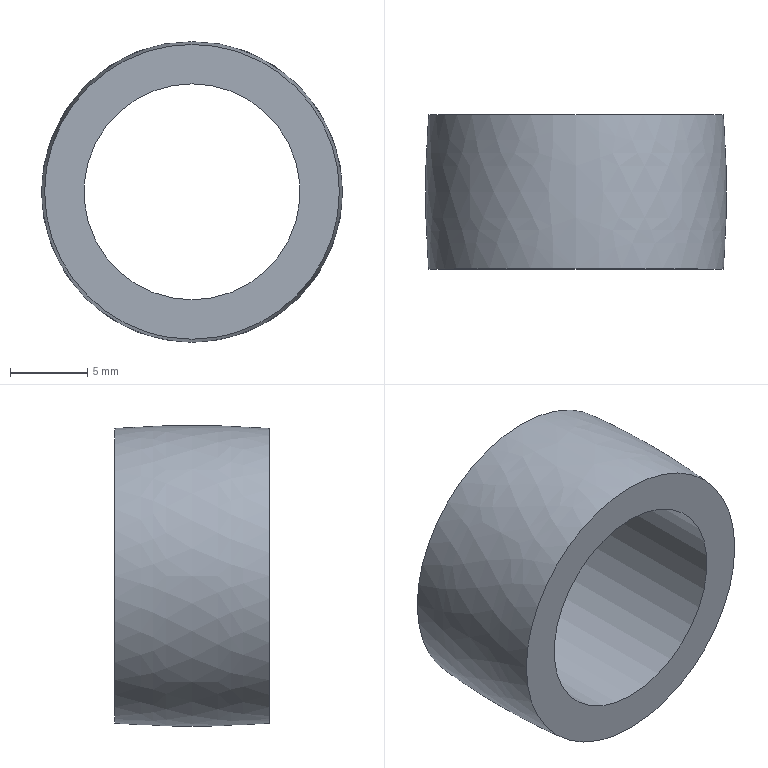Part | STEP file | 1-46.12 | 1 solid | 4 faces | box 19.5 x 10 x 19.5 mm | volume 1406 mm3 | plane 2 | cylinder 1 | spline 1 | commonest cylinder face diameters 14 x1
STEP:
#1=CARTESIAN_POINT('',(0.,0.,0.));
#2=DIRECTION('',(0.,0.,1.));
#3=DIRECTION('',(1.,0.,0.));
#4=AXIS2_PLACEMENT_3D('',#1,#2,#3);
#5=CARTESIAN_POINT('',(0.,0.,7.));
#6=VERTEX_POINT('',#5);
#7=CARTESIAN_POINT('',(0.,0.,0.));
#8=DIRECTION('',(0.,1.,0.));
#9=DIRECTION('',(0.,0.,1.));
#10=AXIS2_PLACEMENT_3D('',#7,#8,#9);
#11=CIRCLE('',#10,7.);
#12=CARTESIAN_POINT('',(0.,0.,0.));
#13=DIRECTION('',(0.,1.,0.));
#14=DIRECTION('',(0.,0.,1.));
#15=AXIS2_PLACEMENT_3D('',#12,#13,#14);
#16=CYLINDRICAL_SURFACE('',#15,7.);
#17=CARTESIAN_POINT('',(0.,0.));
#18=DIRECTION('',(1.,0.));
#19=VECTOR('',#18,1.);
#20=LINE('',#17,#19);
#21=(GEOMETRIC_REPRESENTATION_CONTEXT(2)PARAMETRIC_REPRESENTATION_CONTEXT()REPRESENTATION_CONTEXT('',''));
#22=DEFINITIONAL_REPRESENTATION('',(#20),#21);
#23=PCURVE('',#16,#22);
#24=CARTESIAN_POINT('',(0.,0.,0.));
#25=DIRECTION('',(0.,-1.,0.));
#26=DIRECTION('',(0.,0.,1.));
#27=AXIS2_PLACEMENT_3D('',#24,#25,#26);
#28=PLANE('',#27);
#29=CARTESIAN_POINT('',(7.,0.));
#30=CARTESIAN_POINT('',(7.,-12.124));
#31=CARTESIAN_POINT('',(-3.5,-6.062));
#32=CARTESIAN_POINT('',(-14.,0.));
#33=CARTESIAN_POINT('',(-3.5,6.062));
#34=CARTESIAN_POINT('',(7.,12.124));
#35=CARTESIAN_POINT('',(7.,0.));
#36=(BOUNDED_CURVE()B_SPLINE_CURVE(2,(#29,#30,#31,#32,#33,#34,#35),.UNSPECIFIED.,.T.,.F.)B_SPLINE_CURVE_WITH_KNOTS((1,2,2,2,2,1),(-2.094,0.,2.094,4.189,6.283,8.378),.UNSPECIFIED.)CURVE()GEOMETRIC_REPRESENTATION_ITEM()RATIONAL_B_SPLINE_CURVE((1.,0.5,1.,0.5,1.,0.5,1.))REPRESENTATION_ITEM(''));
#37=(GEOMETRIC_REPRESENTATION_CONTEXT(2)PARAMETRIC_REPRESENTATION_CONTEXT()REPRESENTATION_CONTEXT('',''));
#38=DEFINITIONAL_REPRESENTATION('',(#36),#37);
#39=PCURVE('',#28,#38);
#40=SURFACE_CURVE('',#11,(#23,#39),.PCURVE_S1.);
#41=EDGE_CURVE('',#6,#6,#40,.T.);
#42=ORIENTED_EDGE('',*,*,#41,.T.);
#43=CARTESIAN_POINT('',(0.,10.,7.));
#44=VERTEX_POINT('',#43);
#45=CARTESIAN_POINT('',(0.,0.,7.));
#46=DIRECTION('',(0.,1.,0.));
#47=VECTOR('',#46,1.);
#48=LINE('',#45,#47);
#49=CARTESIAN_POINT('',(6.283,0.));
#50=DIRECTION('',(0.,1.));
#51=VECTOR('',#50,1.);
#52=LINE('',#49,#51);
#53=(GEOMETRIC_REPRESENTATION_CONTEXT(2)PARAMETRIC_REPRESENTATION_CONTEXT()REPRESENTATION_CONTEXT('',''));
#54=DEFINITIONAL_REPRESENTATION('',(#52),#53);
#55=PCURVE('',#16,#54);
#56=CARTESIAN_POINT('',(0.,0.));
#57=DIRECTION('',(0.,1.));
#58=VECTOR('',#57,1.);
#59=LINE('',#56,#58);
#60=(GEOMETRIC_REPRESENTATION_CONTEXT(2)PARAMETRIC_REPRESENTATION_CONTEXT()REPRESENTATION_CONTEXT('',''));
#61=DEFINITIONAL_REPRESENTATION('',(#59),#60);
#62=PCURVE('',#16,#61);
#63=SEAM_CURVE('',#48,(#55,#62),.PCURVE_S1.);
#64=EDGE_CURVE('',#6,#44,#63,.T.);
#65=ORIENTED_EDGE('',*,*,#64,.T.);
#66=CARTESIAN_POINT('',(0.,10.,0.));
#67=DIRECTION('',(0.,1.,0.));
#68=DIRECTION('',(0.,0.,1.));
#69=AXIS2_PLACEMENT_3D('',#66,#67,#68);
#70=CIRCLE('',#69,7.);
#71=CARTESIAN_POINT('',(0.,10.));
#72=DIRECTION('',(1.,0.));
#73=VECTOR('',#72,1.);
#74=LINE('',#71,#73);
#75=(GEOMETRIC_REPRESENTATION_CONTEXT(2)PARAMETRIC_REPRESENTATION_CONTEXT()REPRESENTATION_CONTEXT('',''));
#76=DEFINITIONAL_REPRESENTATION('',(#74),#75);
#77=PCURVE('',#16,#76);
#78=CARTESIAN_POINT('',(0.,10.,0.));
#79=DIRECTION('',(0.,1.,0.));
#80=DIRECTION('',(0.,0.,1.));
#81=AXIS2_PLACEMENT_3D('',#78,#79,#80);
#82=PLANE('',#81);
#83=CARTESIAN_POINT('',(0.,0.));
#84=DIRECTION('',(1.,0.));
#85=AXIS2_PLACEMENT_2D('',#83,#84);
#86=CIRCLE('',#85,7.);
#87=(GEOMETRIC_REPRESENTATION_CONTEXT(2)PARAMETRIC_REPRESENTATION_CONTEXT()REPRESENTATION_CONTEXT('',''));
#88=DEFINITIONAL_REPRESENTATION('',(#86),#87);
#89=PCURVE('',#82,#88);
#90=SURFACE_CURVE('',#70,(#77,#89),.PCURVE_S1.);
#91=EDGE_CURVE('',#44,#44,#90,.T.);
#92=ORIENTED_EDGE('',*,*,#91,.F.);
#93=ORIENTED_EDGE('',*,*,#64,.F.);
#94=EDGE_LOOP('',(#42,#65,#92,#93));
#95=FACE_BOUND('',#94,.F.);
#96=ADVANCED_FACE('',(#95),#16,.F.);
#97=CARTESIAN_POINT('',(0.,10.,9.55));
#98=VERTEX_POINT('',#97);
#99=CARTESIAN_POINT('',(0.,10.,0.));
#100=DIRECTION('',(0.,1.,0.));
#101=DIRECTION('',(0.,0.,1.));
#102=AXIS2_PLACEMENT_3D('',#99,#100,#101);
#103=CIRCLE('',#102,9.55);
#104=CARTESIAN_POINT('',(0.,0.));
#105=DIRECTION('',(1.,0.));
#106=AXIS2_PLACEMENT_2D('',#104,#105);
#107=CIRCLE('',#106,9.55);
#108=(GEOMETRIC_REPRESENTATION_CONTEXT(2)PARAMETRIC_REPRESENTATION_CONTEXT()REPRESENTATION_CONTEXT('',''));
#109=DEFINITIONAL_REPRESENTATION('',(#107),#108);
#110=PCURVE('',#82,#109);
#111=CARTESIAN_POINT('',(0.,10.,9.55));
#112=CARTESIAN_POINT('',(9.55,10.,9.55));
#113=CARTESIAN_POINT('',(9.55,10.,0.));
#114=CARTESIAN_POINT('',(9.55,10.,-9.55));
#115=CARTESIAN_POINT('',(0.,10.,-9.55));
#116=CARTESIAN_POINT('',(-9.55,10.,-9.55));
#117=CARTESIAN_POINT('',(-9.55,10.,0.));
#118=CARTESIAN_POINT('',(-9.55,10.,9.55));
#119=CARTESIAN_POINT('',(0.,10.,9.55));
#120=CARTESIAN_POINT('',(0.,5.,9.951));
#121=CARTESIAN_POINT('',(9.951,5.,9.951));
#122=CARTESIAN_POINT('',(9.951,5.,0.));
#123=CARTESIAN_POINT('',(9.951,5.,-9.951));
#124=CARTESIAN_POINT('',(0.,5.,-9.951));
#125=CARTESIAN_POINT('',(-9.951,5.,-9.951));
#126=CARTESIAN_POINT('',(-9.951,5.,0.));
#127=CARTESIAN_POINT('',(-9.951,5.,9.951));
#128=CARTESIAN_POINT('',(0.,5.,9.951));
#129=CARTESIAN_POINT('',(0.,0.,9.55));
#130=CARTESIAN_POINT('',(9.55,0.,9.55));
#131=CARTESIAN_POINT('',(9.55,0.,0.));
#132=CARTESIAN_POINT('',(9.55,0.,-9.55));
#133=CARTESIAN_POINT('',(0.,0.,-9.55));
#134=CARTESIAN_POINT('',(-9.55,0.,-9.55));
#135=CARTESIAN_POINT('',(-9.55,0.,0.));
#136=CARTESIAN_POINT('',(-9.55,0.,9.55));
#137=CARTESIAN_POINT('',(0.,0.,9.55));
#138=(BOUNDED_SURFACE()B_SPLINE_SURFACE(2,2,((#111,#112,#113,#114,#115,#116,#117,#118,#119),(#120,#121,#122,#123,#124,#125,#126,#127,#128),(#129,#130,#131,#132,#133,#134,#135,#136,#137)),.UNSPECIFIED.,.F.,.T.,.F.)B_SPLINE_SURFACE_WITH_KNOTS((3,3),(1,2,2,2,2,2,1),(0.,1.),(-0.25,0.,0.25,0.5,0.75,1.,1.25),.UNSPECIFIED.)GEOMETRIC_REPRESENTATION_ITEM()RATIONAL_B_SPLINE_SURFACE(((1.,0.7071,1.,0.7071,1.,0.7071,1.,0.7071,1.),(0.9968,0.7048,0.9968,0.7048,0.9968,0.7048,0.9968,0.7048,0.9968),(1.,0.7071,1.,0.7071,1.,0.7071,1.,0.7071,1.)))REPRESENTATION_ITEM('')SURFACE());
#139=CARTESIAN_POINT('',(0.,0.));
#140=CARTESIAN_POINT('',(0.,0.01678));
#141=CARTESIAN_POINT('',(0.,0.04854));
#142=CARTESIAN_POINT('',(0.,0.09277));
#143=CARTESIAN_POINT('',(0.,0.1357));
#144=CARTESIAN_POINT('',(0.,0.1791));
#145=CARTESIAN_POINT('',(0.,0.2245));
#146=CARTESIAN_POINT('',(0.,0.2755));
#147=CARTESIAN_POINT('',(0.,0.3209));
#148=CARTESIAN_POINT('',(0.,0.3643));
#149=CARTESIAN_POINT('',(0.,0.4073));
#150=CARTESIAN_POINT('',(0.,0.4512));
#151=CARTESIAN_POINT('',(0.,0.5));
#152=CARTESIAN_POINT('',(0.,0.5488));
#153=CARTESIAN_POINT('',(0.,0.5927));
#154=CARTESIAN_POINT('',(0.,0.6357));
#155=CARTESIAN_POINT('',(0.,0.6791));
#156=CARTESIAN_POINT('',(0.,0.7245));
#157=CARTESIAN_POINT('',(0.,0.7755));
#158=CARTESIAN_POINT('',(0.,0.8209));
#159=CARTESIAN_POINT('',(0.,0.8643));
#160=CARTESIAN_POINT('',(0.,0.9072));
#161=CARTESIAN_POINT('',(0.,0.9515));
#162=CARTESIAN_POINT('',(0.,0.9832));
#163=CARTESIAN_POINT('',(0.,1.));
#164=B_SPLINE_CURVE_WITH_KNOTS('',3,(#139,#140,#141,#142,#143,#144,#145,#146,#147,#148,#149,#150,#151,#152,#153,#154,#155,#156,#157,#158,#159,#160,#161,#162,#163),.UNSPECIFIED.,.F.,.F.,(4,1,1,1,1,1,1,1,1,1,1,1,1,1,1,1,1,1,1,1,1,1,4),(0.,0.2856,0.5712,0.8568,1.142,1.428,1.714,1.999,2.285,2.57,2.856,3.142,3.427,3.713,3.998,4.284,4.57,4.855,5.141,5.426,5.712,5.998,6.283),.QUASI_UNIFORM_KNOTS.);
#165=(GEOMETRIC_REPRESENTATION_CONTEXT(2)PARAMETRIC_REPRESENTATION_CONTEXT()REPRESENTATION_CONTEXT('',''));
#166=DEFINITIONAL_REPRESENTATION('',(#164),#165);
#167=PCURVE('',#138,#166);
#168=SURFACE_CURVE('',#103,(#110,#167),.PCURVE_S1.);
#169=EDGE_CURVE('',#98,#98,#168,.T.);
#170=ORIENTED_EDGE('',*,*,#169,.T.);
#171=EDGE_LOOP('',(#170));
#172=FACE_BOUND('',#171,.T.);
#173=ORIENTED_EDGE('',*,*,#91,.F.);
#174=EDGE_LOOP('',(#173));
#175=FACE_BOUND('',#174,.T.);
#176=ADVANCED_FACE('',(#172,#175),#82,.T.);
#177=CARTESIAN_POINT('',(0.,0.,9.55));
#178=VERTEX_POINT('',#177);
#179=CARTESIAN_POINT('',(0.,5.,-52.85));
#180=DIRECTION('',(1.,0.,0.));
#181=DIRECTION('',(0.,0.07987,0.9968));
#182=AXIS2_PLACEMENT_3D('',#179,#180,#181);
#183=CIRCLE('',#182,62.6);
#184=CARTESIAN_POINT('',(0.,0.));
#185=CARTESIAN_POINT('',(1.,0.));
#186=B_SPLINE_CURVE_WITH_KNOTS('',1,(#184,#185),.UNSPECIFIED.,.F.,.F.,(2,2),(0.,0.1599),.PIECEWISE_BEZIER_KNOTS.);
#187=(GEOMETRIC_REPRESENTATION_CONTEXT(2)PARAMETRIC_REPRESENTATION_CONTEXT()REPRESENTATION_CONTEXT('',''));
#188=DEFINITIONAL_REPRESENTATION('',(#186),#187);
#189=PCURVE('',#138,#188);
#190=CARTESIAN_POINT('',(0.,1.));
#191=CARTESIAN_POINT('',(1.,1.));
#192=B_SPLINE_CURVE_WITH_KNOTS('',1,(#190,#191),.UNSPECIFIED.,.F.,.F.,(2,2),(0.,0.1599),.PIECEWISE_BEZIER_KNOTS.);
#193=(GEOMETRIC_REPRESENTATION_CONTEXT(2)PARAMETRIC_REPRESENTATION_CONTEXT()REPRESENTATION_CONTEXT('',''));
#194=DEFINITIONAL_REPRESENTATION('',(#192),#193);
#195=PCURVE('',#138,#194);
#196=SEAM_CURVE('',#183,(#189,#195),.PCURVE_S1.);
#197=EDGE_CURVE('',#98,#178,#196,.T.);
#198=ORIENTED_EDGE('',*,*,#197,.T.);
#199=CARTESIAN_POINT('',(0.,0.,0.));
#200=DIRECTION('',(0.,1.,0.));
#201=DIRECTION('',(0.,0.,1.));
#202=AXIS2_PLACEMENT_3D('',#199,#200,#201);
#203=CIRCLE('',#202,9.55);
#204=CARTESIAN_POINT('',(1.,0.));
#205=CARTESIAN_POINT('',(1.,0.01678));
#206=CARTESIAN_POINT('',(1.,0.04854));
#207=CARTESIAN_POINT('',(1.,0.09277));
#208=CARTESIAN_POINT('',(1.,0.1357));
#209=CARTESIAN_POINT('',(1.,0.1791));
#210=CARTESIAN_POINT('',(1.,0.2245));
#211=CARTESIAN_POINT('',(1.,0.2755));
#212=CARTESIAN_POINT('',(1.,0.3209));
#213=CARTESIAN_POINT('',(1.,0.3643));
#214=CARTESIAN_POINT('',(1.,0.4073));
#215=CARTESIAN_POINT('',(1.,0.4512));
#216=CARTESIAN_POINT('',(1.,0.5));
#217=CARTESIAN_POINT('',(1.,0.5488));
#218=CARTESIAN_POINT('',(1.,0.5927));
#219=CARTESIAN_POINT('',(1.,0.6357));
#220=CARTESIAN_POINT('',(1.,0.6791));
#221=CARTESIAN_POINT('',(1.,0.7245));
#222=CARTESIAN_POINT('',(1.,0.7755));
#223=CARTESIAN_POINT('',(1.,0.8209));
#224=CARTESIAN_POINT('',(1.,0.8643));
#225=CARTESIAN_POINT('',(1.,0.9072));
#226=CARTESIAN_POINT('',(1.,0.9515));
#227=CARTESIAN_POINT('',(1.,0.9832));
#228=CARTESIAN_POINT('',(1.,1.));
#229=B_SPLINE_CURVE_WITH_KNOTS('',3,(#204,#205,#206,#207,#208,#209,#210,#211,#212,#213,#214,#215,#216,#217,#218,#219,#220,#221,#222,#223,#224,#225,#226,#227,#228),.UNSPECIFIED.,.F.,.F.,(4,1,1,1,1,1,1,1,1,1,1,1,1,1,1,1,1,1,1,1,1,1,4),(0.,0.2856,0.5712,0.8568,1.142,1.428,1.714,1.999,2.285,2.57,2.856,3.142,3.427,3.713,3.998,4.284,4.57,4.855,5.141,5.426,5.712,5.998,6.283),.QUASI_UNIFORM_KNOTS.);
#230=(GEOMETRIC_REPRESENTATION_CONTEXT(2)PARAMETRIC_REPRESENTATION_CONTEXT()REPRESENTATION_CONTEXT('',''));
#231=DEFINITIONAL_REPRESENTATION('',(#229),#230);
#232=PCURVE('',#138,#231);
#233=CARTESIAN_POINT('',(9.55,0.));
#234=CARTESIAN_POINT('',(9.55,-16.541));
#235=CARTESIAN_POINT('',(-4.775,-8.271));
#236=CARTESIAN_POINT('',(-19.1,0.));
#237=CARTESIAN_POINT('',(-4.775,8.271));
#238=CARTESIAN_POINT('',(9.55,16.541));
#239=CARTESIAN_POINT('',(9.55,0.));
#240=(BOUNDED_CURVE()B_SPLINE_CURVE(2,(#233,#234,#235,#236,#237,#238,#239),.UNSPECIFIED.,.T.,.F.)B_SPLINE_CURVE_WITH_KNOTS((1,2,2,2,2,1),(-2.094,0.,2.094,4.189,6.283,8.378),.UNSPECIFIED.)CURVE()GEOMETRIC_REPRESENTATION_ITEM()RATIONAL_B_SPLINE_CURVE((1.,0.5,1.,0.5,1.,0.5,1.))REPRESENTATION_ITEM(''));
#241=(GEOMETRIC_REPRESENTATION_CONTEXT(2)PARAMETRIC_REPRESENTATION_CONTEXT()REPRESENTATION_CONTEXT('',''));
#242=DEFINITIONAL_REPRESENTATION('',(#240),#241);
#243=PCURVE('',#28,#242);
#244=SURFACE_CURVE('',#203,(#232,#243),.PCURVE_S1.);
#245=EDGE_CURVE('',#178,#178,#244,.T.);
#246=ORIENTED_EDGE('',*,*,#245,.T.);
#247=ORIENTED_EDGE('',*,*,#197,.F.);
#248=ORIENTED_EDGE('',*,*,#169,.F.);
#249=EDGE_LOOP('',(#198,#246,#247,#248));
#250=FACE_BOUND('',#249,.T.);
#251=ADVANCED_FACE('',(#250),#138,.T.);
#252=ORIENTED_EDGE('',*,*,#245,.F.);
#253=EDGE_LOOP('',(#252));
#254=FACE_BOUND('',#253,.T.);
#255=ORIENTED_EDGE('',*,*,#41,.T.);
#256=EDGE_LOOP('',(#255));
#257=FACE_BOUND('',#256,.T.);
#258=ADVANCED_FACE('',(#254,#257),#28,.T.);
#259=CLOSED_SHELL('',(#96,#176,#251,#258));
#260=MANIFOLD_SOLID_BREP('',#259);
#261=(LENGTH_UNIT()NAMED_UNIT(*)SI_UNIT(.MILLI.,.METRE.));
#262=UNCERTAINTY_MEASURE_WITH_UNIT(LENGTH_MEASURE(0.0005),#261,'','');
#263=(NAMED_UNIT(*)PLANE_ANGLE_UNIT()SI_UNIT($,.RADIAN.));
#264=(NAMED_UNIT(*)SI_UNIT($,.STERADIAN.)SOLID_ANGLE_UNIT());
#265=(GEOMETRIC_REPRESENTATION_CONTEXT(3)GLOBAL_UNCERTAINTY_ASSIGNED_CONTEXT((#262))GLOBAL_UNIT_ASSIGNED_CONTEXT((#261,#263,#264))REPRESENTATION_CONTEXT('',''));
#266=ADVANCED_BREP_SHAPE_REPRESENTATION('',(#4,#260),#265);